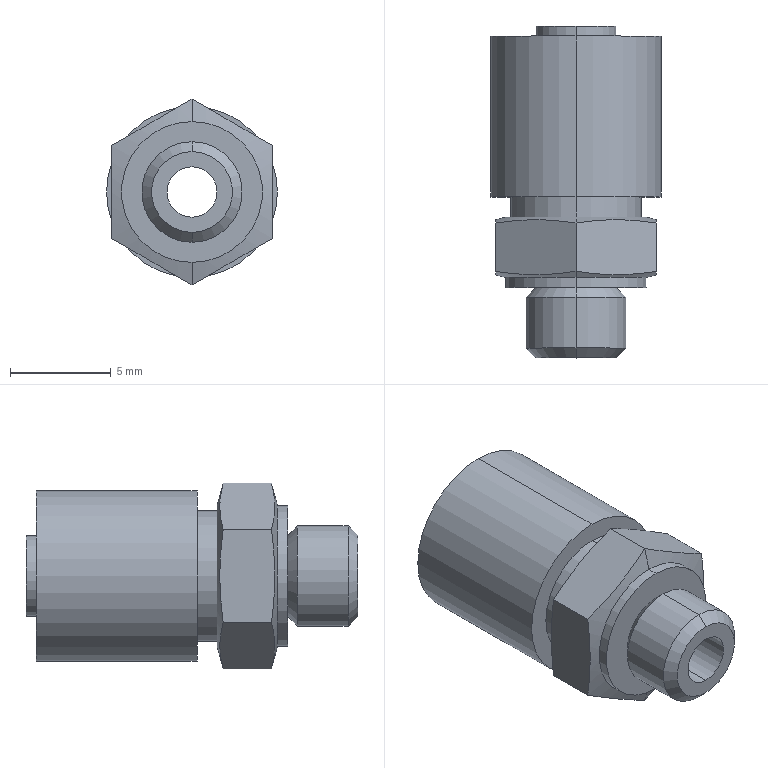Part | SolidWorks | features BaseBody 1 | 1 solid | 32 faces | box 8.5 x 16.5 x 9.238 mm | volume 659.616 mm3 | plane 12 | cylinder 12 | cone 8 | commonest cylinder face diameters 2.5 x2 4 x2 5 x2 6.5 x2 7 x2 8.5 x2
STEP:
#1=CARTESIAN_POINT('',(0.,16.5,-1.25));
#2=VERTEX_POINT('',#1);
#3=CARTESIAN_POINT('',(0.,16.5,1.25));
#4=VERTEX_POINT('',#3);
#5=CARTESIAN_POINT('',(0.,16.5,0.));
#6=DIRECTION('',(0.,-1.,0.));
#7=DIRECTION('',(0.,0.,-1.));
#8=AXIS2_PLACEMENT_3D('',#5,#6,#7);
#9=CIRCLE('',#8,1.25);
#10=EDGE_CURVE('',#2,#4,#9,.T.);
#11=ORIENTED_EDGE('',*,*,#10,.T.);
#12=CARTESIAN_POINT('',(0.,16.5,0.));
#13=DIRECTION('',(0.,-1.,0.));
#14=DIRECTION('',(0.,0.,-1.));
#15=AXIS2_PLACEMENT_3D('',#12,#13,#14);
#16=CIRCLE('',#15,1.25);
#17=EDGE_CURVE('',#4,#2,#16,.T.);
#18=ORIENTED_EDGE('',*,*,#17,.T.);
#19=EDGE_LOOP('',(#11,#18));
#20=FACE_BOUND('',#19,.T.);
#21=CARTESIAN_POINT('',(0.,16.5,-2.));
#22=VERTEX_POINT('',#21);
#23=CARTESIAN_POINT('',(0.,16.5,2.));
#24=VERTEX_POINT('',#23);
#25=CARTESIAN_POINT('',(0.,16.5,0.));
#26=DIRECTION('',(0.,-1.,0.));
#27=DIRECTION('',(0.,0.,-1.));
#28=AXIS2_PLACEMENT_3D('',#25,#26,#27);
#29=CIRCLE('',#28,2.);
#30=EDGE_CURVE('',#22,#24,#29,.T.);
#31=ORIENTED_EDGE('',*,*,#30,.F.);
#32=CARTESIAN_POINT('',(0.,16.5,0.));
#33=DIRECTION('',(0.,-1.,0.));
#34=DIRECTION('',(0.,0.,-1.));
#35=AXIS2_PLACEMENT_3D('',#32,#33,#34);
#36=CIRCLE('',#35,2.);
#37=EDGE_CURVE('',#24,#22,#36,.T.);
#38=ORIENTED_EDGE('',*,*,#37,.F.);
#39=EDGE_LOOP('',(#31,#38));
#40=FACE_OUTER_BOUND('',#39,.T.);
#41=CARTESIAN_POINT('',(2.,16.5,0.));
#42=DIRECTION('',(0.,1.,0.));
#43=DIRECTION('',(1.,0.,0.));
#44=AXIS2_PLACEMENT_3D('',#41,#42,#43);
#45=PLANE('',#44);
#46=ADVANCED_FACE('',(#20,#40),#45,.T.);
#47=CARTESIAN_POINT('',(0.,0.,1.25));
#48=VERTEX_POINT('',#47);
#49=CARTESIAN_POINT('',(0.,0.,1.25));
#50=DIRECTION('',(0.,-1.,0.));
#51=VECTOR('',#50,1000.);
#52=LINE('',#49,#51);
#53=EDGE_CURVE('',#4,#48,#52,.T.);
#54=ORIENTED_EDGE('',*,*,#53,.F.);
#55=ORIENTED_EDGE('',*,*,#10,.F.);
#56=CARTESIAN_POINT('',(0.,0.,-1.25));
#57=VERTEX_POINT('',#56);
#58=CARTESIAN_POINT('',(0.,0.,-1.25));
#59=DIRECTION('',(0.,-1.,0.));
#60=VECTOR('',#59,1000.);
#61=LINE('',#58,#60);
#62=EDGE_CURVE('',#2,#57,#61,.T.);
#63=ORIENTED_EDGE('',*,*,#62,.T.);
#64=CARTESIAN_POINT('',(0.,0.,0.));
#65=DIRECTION('',(0.,-1.,0.));
#66=DIRECTION('',(0.,0.,-1.));
#67=AXIS2_PLACEMENT_3D('',#64,#65,#66);
#68=CIRCLE('',#67,1.25);
#69=EDGE_CURVE('',#57,#48,#68,.T.);
#70=ORIENTED_EDGE('',*,*,#69,.T.);
#71=EDGE_LOOP('',(#54,#55,#63,#70));
#72=FACE_OUTER_BOUND('',#71,.T.);
#73=CARTESIAN_POINT('',(0.,0.,0.));
#74=DIRECTION('',(0.,-1.,0.));
#75=DIRECTION('',(0.,0.,-1.));
#76=AXIS2_PLACEMENT_3D('',#73,#74,#75);
#77=CYLINDRICAL_SURFACE('',#76,1.25);
#78=ADVANCED_FACE('',(#72),#77,.F.);
#79=ORIENTED_EDGE('',*,*,#69,.F.);
#80=CARTESIAN_POINT('',(0.,0.,0.));
#81=DIRECTION('',(0.,-1.,0.));
#82=DIRECTION('',(0.,0.,-1.));
#83=AXIS2_PLACEMENT_3D('',#80,#81,#82);
#84=CIRCLE('',#83,1.25);
#85=EDGE_CURVE('',#48,#57,#84,.T.);
#86=ORIENTED_EDGE('',*,*,#85,.F.);
#87=EDGE_LOOP('',(#79,#86));
#88=FACE_BOUND('',#87,.T.);
#89=CARTESIAN_POINT('',(0.,0.,2.01));
#90=VERTEX_POINT('',#89);
#91=CARTESIAN_POINT('',(0.,0.,-2.01));
#92=VERTEX_POINT('',#91);
#93=CARTESIAN_POINT('',(0.,0.,0.));
#94=DIRECTION('',(0.,-1.,0.));
#95=DIRECTION('',(0.,0.,-1.));
#96=AXIS2_PLACEMENT_3D('',#93,#94,#95);
#97=CIRCLE('',#96,2.01);
#98=EDGE_CURVE('',#90,#92,#97,.T.);
#99=ORIENTED_EDGE('',*,*,#98,.T.);
#100=CARTESIAN_POINT('',(0.,0.,0.));
#101=DIRECTION('',(0.,-1.,0.));
#102=DIRECTION('',(0.,0.,-1.));
#103=AXIS2_PLACEMENT_3D('',#100,#101,#102);
#104=CIRCLE('',#103,2.01);
#105=EDGE_CURVE('',#92,#90,#104,.T.);
#106=ORIENTED_EDGE('',*,*,#105,.T.);
#107=EDGE_LOOP('',(#99,#106));
#108=FACE_OUTER_BOUND('',#107,.T.);
#109=CARTESIAN_POINT('',(1.25,0.,0.));
#110=DIRECTION('',(0.,-1.,0.));
#111=DIRECTION('',(0.,0.,-1.));
#112=AXIS2_PLACEMENT_3D('',#109,#110,#111);
#113=PLANE('',#112);
#114=ADVANCED_FACE('',(#88,#108),#113,.T.);
#115=CARTESIAN_POINT('',(0.,0.4905,-2.5));
#116=VERTEX_POINT('',#115);
#117=CARTESIAN_POINT('',(0.,0.,-2.01));
#118=DIRECTION('',(0.,0.7071,-0.7071));
#119=VECTOR('',#118,1000.);
#120=LINE('',#117,#119);
#121=EDGE_CURVE('',#92,#116,#120,.T.);
#122=ORIENTED_EDGE('',*,*,#121,.F.);
#123=ORIENTED_EDGE('',*,*,#98,.F.);
#124=CARTESIAN_POINT('',(0.,0.4905,2.5));
#125=VERTEX_POINT('',#124);
#126=CARTESIAN_POINT('',(0.,0.,2.01));
#127=DIRECTION('',(0.,0.7071,0.7071));
#128=VECTOR('',#127,1000.);
#129=LINE('',#126,#128);
#130=EDGE_CURVE('',#90,#125,#129,.T.);
#131=ORIENTED_EDGE('',*,*,#130,.T.);
#132=CARTESIAN_POINT('',(0.,0.4905,0.));
#133=DIRECTION('',(0.,-1.,0.));
#134=DIRECTION('',(0.,0.,-1.));
#135=AXIS2_PLACEMENT_3D('',#132,#133,#134);
#136=CIRCLE('',#135,2.5);
#137=EDGE_CURVE('',#125,#116,#136,.T.);
#138=ORIENTED_EDGE('',*,*,#137,.T.);
#139=EDGE_LOOP('',(#122,#123,#131,#138));
#140=FACE_OUTER_BOUND('',#139,.T.);
#141=CARTESIAN_POINT('',(0.,0.,0.));
#142=DIRECTION('',(0.,1.,0.));
#143=DIRECTION('',(0.,0.,1.));
#144=AXIS2_PLACEMENT_3D('',#141,#142,#143);
#145=CONICAL_SURFACE('',#144,2.01,0.7854);
#146=ADVANCED_FACE('',(#140),#145,.T.);
#147=CARTESIAN_POINT('',(0.,3.01,2.5));
#148=VERTEX_POINT('',#147);
#149=CARTESIAN_POINT('',(0.,0.,2.5));
#150=DIRECTION('',(0.,-1.,0.));
#151=VECTOR('',#150,1000.);
#152=LINE('',#149,#151);
#153=EDGE_CURVE('',#148,#125,#152,.T.);
#154=ORIENTED_EDGE('',*,*,#153,.F.);
#155=CARTESIAN_POINT('',(0.,3.01,-2.5));
#156=VERTEX_POINT('',#155);
#157=CARTESIAN_POINT('',(0.,3.01,0.));
#158=DIRECTION('',(0.,-1.,0.));
#159=DIRECTION('',(0.,0.,-1.));
#160=AXIS2_PLACEMENT_3D('',#157,#158,#159);
#161=CIRCLE('',#160,2.5);
#162=EDGE_CURVE('',#148,#156,#161,.T.);
#163=ORIENTED_EDGE('',*,*,#162,.T.);
#164=CARTESIAN_POINT('',(0.,0.,-2.5));
#165=DIRECTION('',(0.,-1.,0.));
#166=VECTOR('',#165,1000.);
#167=LINE('',#164,#166);
#168=EDGE_CURVE('',#156,#116,#167,.T.);
#169=ORIENTED_EDGE('',*,*,#168,.T.);
#170=ORIENTED_EDGE('',*,*,#137,.F.);
#171=EDGE_LOOP('',(#154,#163,#169,#170));
#172=FACE_OUTER_BOUND('',#171,.T.);
#173=CARTESIAN_POINT('',(0.,0.,0.));
#174=DIRECTION('',(0.,-1.,0.));
#175=DIRECTION('',(0.,0.,-1.));
#176=AXIS2_PLACEMENT_3D('',#173,#174,#175);
#177=CYLINDRICAL_SURFACE('',#176,2.5);
#178=ADVANCED_FACE('',(#172),#177,.T.);
#179=CARTESIAN_POINT('',(0.,3.5,2.01));
#180=VERTEX_POINT('',#179);
#181=CARTESIAN_POINT('',(0.,3.01,2.5));
#182=DIRECTION('',(0.,-0.7071,0.7071));
#183=VECTOR('',#182,1000.);
#184=LINE('',#181,#183);
#185=EDGE_CURVE('',#180,#148,#184,.T.);
#186=ORIENTED_EDGE('',*,*,#185,.F.);
#187=CARTESIAN_POINT('',(0.,3.5,-2.01));
#188=VERTEX_POINT('',#187);
#189=CARTESIAN_POINT('',(0.,3.5,0.));
#190=DIRECTION('',(0.,-1.,0.));
#191=DIRECTION('',(0.,0.,-1.));
#192=AXIS2_PLACEMENT_3D('',#189,#190,#191);
#193=CIRCLE('',#192,2.01);
#194=EDGE_CURVE('',#180,#188,#193,.T.);
#195=ORIENTED_EDGE('',*,*,#194,.T.);
#196=CARTESIAN_POINT('',(0.,3.01,-2.5));
#197=DIRECTION('',(0.,-0.7071,-0.7071));
#198=VECTOR('',#197,1000.);
#199=LINE('',#196,#198);
#200=EDGE_CURVE('',#188,#156,#199,.T.);
#201=ORIENTED_EDGE('',*,*,#200,.T.);
#202=ORIENTED_EDGE('',*,*,#162,.F.);
#203=EDGE_LOOP('',(#186,#195,#201,#202));
#204=FACE_OUTER_BOUND('',#203,.T.);
#205=CARTESIAN_POINT('',(0.,3.01,0.));
#206=DIRECTION('',(0.,-1.,0.));
#207=DIRECTION('',(0.,0.,-1.));
#208=AXIS2_PLACEMENT_3D('',#205,#206,#207);
#209=CONICAL_SURFACE('',#208,2.5,0.7854);
#210=ADVANCED_FACE('',(#204),#209,.T.);
#211=CARTESIAN_POINT('',(0.,3.5,0.));
#212=DIRECTION('',(0.,-1.,0.));
#213=DIRECTION('',(0.,0.,-1.));
#214=AXIS2_PLACEMENT_3D('',#211,#212,#213);
#215=CIRCLE('',#214,2.01);
#216=EDGE_CURVE('',#188,#180,#215,.T.);
#217=ORIENTED_EDGE('',*,*,#216,.F.);
#218=ORIENTED_EDGE('',*,*,#194,.F.);
#219=EDGE_LOOP('',(#217,#218));
#220=FACE_BOUND('',#219,.T.);
#221=CARTESIAN_POINT('',(0.,3.5,-3.5));
#222=VERTEX_POINT('',#221);
#223=CARTESIAN_POINT('',(0.,3.5,3.5));
#224=VERTEX_POINT('',#223);
#225=CARTESIAN_POINT('',(0.,3.5,0.));
#226=DIRECTION('',(0.,-1.,0.));
#227=DIRECTION('',(0.,0.,-1.));
#228=AXIS2_PLACEMENT_3D('',#225,#226,#227);
#229=CIRCLE('',#228,3.5);
#230=EDGE_CURVE('',#222,#224,#229,.T.);
#231=ORIENTED_EDGE('',*,*,#230,.T.);
#232=CARTESIAN_POINT('',(0.,3.5,0.));
#233=DIRECTION('',(0.,-1.,0.));
#234=DIRECTION('',(0.,0.,-1.));
#235=AXIS2_PLACEMENT_3D('',#232,#233,#234);
#236=CIRCLE('',#235,3.5);
#237=EDGE_CURVE('',#224,#222,#236,.T.);
#238=ORIENTED_EDGE('',*,*,#237,.T.);
#239=EDGE_LOOP('',(#231,#238));
#240=FACE_OUTER_BOUND('',#239,.T.);
#241=CARTESIAN_POINT('',(2.01,3.5,0.));
#242=DIRECTION('',(0.,-1.,0.));
#243=DIRECTION('',(0.,0.,-1.));
#244=AXIS2_PLACEMENT_3D('',#241,#242,#243);
#245=PLANE('',#244);
#246=ADVANCED_FACE('',(#220,#240),#245,.T.);
#247=CARTESIAN_POINT('',(0.,4.,3.5));
#248=VERTEX_POINT('',#247);
#249=CARTESIAN_POINT('',(0.,0.,3.5));
#250=DIRECTION('',(0.,-1.,0.));
#251=VECTOR('',#250,1000.);
#252=LINE('',#249,#251);
#253=EDGE_CURVE('',#248,#224,#252,.T.);
#254=ORIENTED_EDGE('',*,*,#253,.F.);
#255=CARTESIAN_POINT('',(0.,4.,-3.5));
#256=VERTEX_POINT('',#255);
#257=CARTESIAN_POINT('',(0.,4.,0.));
#258=DIRECTION('',(0.,-1.,0.));
#259=DIRECTION('',(0.,0.,-1.));
#260=AXIS2_PLACEMENT_3D('',#257,#258,#259);
#261=CIRCLE('',#260,3.5);
#262=EDGE_CURVE('',#248,#256,#261,.T.);
#263=ORIENTED_EDGE('',*,*,#262,.T.);
#264=CARTESIAN_POINT('',(0.,0.,-3.5));
#265=DIRECTION('',(0.,-1.,0.));
#266=VECTOR('',#265,1000.);
#267=LINE('',#264,#266);
#268=EDGE_CURVE('',#256,#222,#267,.T.);
#269=ORIENTED_EDGE('',*,*,#268,.T.);
#270=ORIENTED_EDGE('',*,*,#237,.F.);
#271=EDGE_LOOP('',(#254,#263,#269,#270));
#272=FACE_OUTER_BOUND('',#271,.T.);
#273=CARTESIAN_POINT('',(0.,0.,0.));
#274=DIRECTION('',(0.,-1.,0.));
#275=DIRECTION('',(0.,0.,-1.));
#276=AXIS2_PLACEMENT_3D('',#273,#274,#275);
#277=CYLINDRICAL_SURFACE('',#276,3.5);
#278=ADVANCED_FACE('',(#272),#277,.T.);
#279=CARTESIAN_POINT('',(0.,4.3,-4.619));
#280=VERTEX_POINT('',#279);
#281=CARTESIAN_POINT('',(0.,4.,-3.5));
#282=DIRECTION('',(0.,0.2588,-0.9659));
#283=VECTOR('',#282,1000.);
#284=LINE('',#281,#283);
#285=EDGE_CURVE('',#256,#280,#284,.T.);
#286=ORIENTED_EDGE('',*,*,#285,.F.);
#287=ORIENTED_EDGE('',*,*,#262,.F.);
#288=CARTESIAN_POINT('',(0.,4.3,4.619));
#289=VERTEX_POINT('',#288);
#290=CARTESIAN_POINT('',(0.,4.,3.5));
#291=DIRECTION('',(0.,0.2588,0.9659));
#292=VECTOR('',#291,1000.);
#293=LINE('',#290,#292);
#294=EDGE_CURVE('',#248,#289,#293,.T.);
#295=ORIENTED_EDGE('',*,*,#294,.T.);
#296=CARTESIAN_POINT('',(-4.,4.3,2.309));
#297=VERTEX_POINT('',#296);
#298=CARTESIAN_POINT('',(-4.,4.3,2.309));
#299=CARTESIAN_POINT('',(-3.286,4.189,2.722));
#300=CARTESIAN_POINT('',(-2.618,4.134,3.107));
#301=CARTESIAN_POINT('',(-1.382,4.134,3.821));
#302=CARTESIAN_POINT('',(-0.7149,4.189,4.206));
#303=CARTESIAN_POINT('',(0.,4.3,4.619));
#304=B_SPLINE_CURVE_WITH_KNOTS('',3,(#298,#299,#300,#301,#302,#303),.UNSPECIFIED.,.F.,.F.,(4,2,4),(0.,0.5,1.),.UNSPECIFIED.);
#305=EDGE_CURVE('',#297,#289,#304,.T.);
#306=ORIENTED_EDGE('',*,*,#305,.F.);
#307=CARTESIAN_POINT('',(-4.,4.3,-2.309));
#308=VERTEX_POINT('',#307);
#309=CARTESIAN_POINT('',(-4.,4.3,-2.309));
#310=CARTESIAN_POINT('',(-4.,4.245,-1.899));
#311=CARTESIAN_POINT('',(-4.,4.183,-1.304));
#312=CARTESIAN_POINT('',(-4.,4.146,-0.6473));
#313=CARTESIAN_POINT('',(-4.,4.138,-0.3741));
#314=CARTESIAN_POINT('',(-4.,4.135,-0.1937));
#315=CARTESIAN_POINT('',(-4.,4.134,-0.1062));
#316=CARTESIAN_POINT('',(-4.,4.134,0.7059));
#317=CARTESIAN_POINT('',(-4.,4.189,1.481));
#318=CARTESIAN_POINT('',(-4.,4.3,2.309));
#319=B_SPLINE_CURVE_WITH_KNOTS('',3,(#309,#310,#311,#312,#313,#314,#315,#316,#317,#318),.UNSPECIFIED.,.F.,.F.,(4,1,1,2,2,4),(0.,0.25,0.375,0.4375,0.5,1.),.UNSPECIFIED.);
#320=EDGE_CURVE('',#308,#297,#319,.T.);
#321=ORIENTED_EDGE('',*,*,#320,.F.);
#322=CARTESIAN_POINT('',(0.,4.3,-4.619));
#323=CARTESIAN_POINT('',(-0.7142,4.189,-4.206));
#324=CARTESIAN_POINT('',(-1.382,4.134,-3.821));
#325=CARTESIAN_POINT('',(-2.618,4.134,-3.107));
#326=CARTESIAN_POINT('',(-3.285,4.189,-2.722));
#327=CARTESIAN_POINT('',(-4.,4.3,-2.309));
#328=B_SPLINE_CURVE_WITH_KNOTS('',3,(#322,#323,#324,#325,#326,#327),.UNSPECIFIED.,.F.,.F.,(4,2,4),(0.,0.5,1.),.UNSPECIFIED.);
#329=EDGE_CURVE('',#280,#308,#328,.T.);
#330=ORIENTED_EDGE('',*,*,#329,.F.);
#331=EDGE_LOOP('',(#286,#287,#295,#306,#321,#330));
#332=FACE_OUTER_BOUND('',#331,.T.);
#333=CARTESIAN_POINT('',(0.,4.,0.));
#334=DIRECTION('',(0.,1.,0.));
#335=DIRECTION('',(0.,0.,1.));
#336=AXIS2_PLACEMENT_3D('',#333,#334,#335);
#337=CONICAL_SURFACE('',#336,3.5,1.309);
#338=ADVANCED_FACE('',(#332),#337,.T.);
#339=CARTESIAN_POINT('',(0.,7.,3.5));
#340=VERTEX_POINT('',#339);
#341=CARTESIAN_POINT('',(0.,6.7,4.619));
#342=VERTEX_POINT('',#341);
#343=CARTESIAN_POINT('',(0.,5.794,8.));
#344=DIRECTION('',(0.,-0.2588,0.9659));
#345=VECTOR('',#344,1000.);
#346=LINE('',#343,#345);
#347=EDGE_CURVE('',#340,#342,#346,.T.);
#348=ORIENTED_EDGE('',*,*,#347,.F.);
#349=CARTESIAN_POINT('',(0.,7.,-3.5));
#350=VERTEX_POINT('',#349);
#351=CARTESIAN_POINT('',(0.,7.,0.));
#352=DIRECTION('',(0.,-1.,0.));
#353=DIRECTION('',(0.,0.,-1.));
#354=AXIS2_PLACEMENT_3D('',#351,#352,#353);
#355=CIRCLE('',#354,3.5);
#356=EDGE_CURVE('',#340,#350,#355,.T.);
#357=ORIENTED_EDGE('',*,*,#356,.T.);
#358=CARTESIAN_POINT('',(0.,6.7,-4.619));
#359=VERTEX_POINT('',#358);
#360=CARTESIAN_POINT('',(0.,5.794,-8.));
#361=DIRECTION('',(0.,-0.2588,-0.9659));
#362=VECTOR('',#361,1000.);
#363=LINE('',#360,#362);
#364=EDGE_CURVE('',#350,#359,#363,.T.);
#365=ORIENTED_EDGE('',*,*,#364,.T.);
#366=CARTESIAN_POINT('',(-4.,6.7,-2.309));
#367=VERTEX_POINT('',#366);
#368=CARTESIAN_POINT('',(-4.,6.7,-2.309));
#369=CARTESIAN_POINT('',(-3.286,6.811,-2.722));
#370=CARTESIAN_POINT('',(-2.618,6.866,-3.107));
#371=CARTESIAN_POINT('',(-1.382,6.866,-3.821));
#372=CARTESIAN_POINT('',(-0.7149,6.811,-4.206));
#373=CARTESIAN_POINT('',(0.,6.7,-4.619));
#374=B_SPLINE_CURVE_WITH_KNOTS('',3,(#368,#369,#370,#371,#372,#373),.UNSPECIFIED.,.F.,.F.,(4,2,4),(0.,0.5,1.),.UNSPECIFIED.);
#375=EDGE_CURVE('',#367,#359,#374,.T.);
#376=ORIENTED_EDGE('',*,*,#375,.F.);
#377=CARTESIAN_POINT('',(-4.,6.7,2.309));
#378=VERTEX_POINT('',#377);
#379=CARTESIAN_POINT('',(-4.,6.7,2.309));
#380=CARTESIAN_POINT('',(-4.,6.755,1.899));
#381=CARTESIAN_POINT('',(-4.,6.817,1.304));
#382=CARTESIAN_POINT('',(-4.,6.854,0.6473));
#383=CARTESIAN_POINT('',(-4.,6.862,0.3741));
#384=CARTESIAN_POINT('',(-4.,6.865,0.1937));
#385=CARTESIAN_POINT('',(-4.,6.866,0.1062));
#386=CARTESIAN_POINT('',(-4.,6.866,-0.7059));
#387=CARTESIAN_POINT('',(-4.,6.811,-1.481));
#388=CARTESIAN_POINT('',(-4.,6.7,-2.309));
#389=B_SPLINE_CURVE_WITH_KNOTS('',3,(#379,#380,#381,#382,#383,#384,#385,#386,#387,#388),.UNSPECIFIED.,.F.,.F.,(4,1,1,2,2,4),(0.,0.25,0.375,0.4375,0.5,1.),.UNSPECIFIED.);
#390=EDGE_CURVE('',#378,#367,#389,.T.);
#391=ORIENTED_EDGE('',*,*,#390,.F.);
#392=CARTESIAN_POINT('',(0.,6.7,4.619));
#393=CARTESIAN_POINT('',(-0.7142,6.811,4.206));
#394=CARTESIAN_POINT('',(-1.382,6.866,3.821));
#395=CARTESIAN_POINT('',(-2.618,6.866,3.107));
#396=CARTESIAN_POINT('',(-3.285,6.811,2.722));
#397=CARTESIAN_POINT('',(-4.,6.7,2.309));
#398=B_SPLINE_CURVE_WITH_KNOTS('',3,(#392,#393,#394,#395,#396,#397),.UNSPECIFIED.,.F.,.F.,(4,2,4),(0.,0.5,1.),.UNSPECIFIED.);
#399=EDGE_CURVE('',#342,#378,#398,.T.);
#400=ORIENTED_EDGE('',*,*,#399,.F.);
#401=EDGE_LOOP('',(#348,#357,#365,#376,#391,#400));
#402=FACE_OUTER_BOUND('',#401,.T.);
#403=CARTESIAN_POINT('',(0.,5.794,0.));
#404=DIRECTION('',(0.,-1.,0.));
#405=DIRECTION('',(0.,0.,-1.));
#406=AXIS2_PLACEMENT_3D('',#403,#404,#405);
#407=CONICAL_SURFACE('',#406,8.,1.309);
#408=ADVANCED_FACE('',(#402),#407,.T.);
#409=CARTESIAN_POINT('',(0.,7.,-3.25));
#410=VERTEX_POINT('',#409);
#411=CARTESIAN_POINT('',(0.,7.,3.25));
#412=VERTEX_POINT('',#411);
#413=CARTESIAN_POINT('',(0.,7.,0.));
#414=DIRECTION('',(0.,-1.,0.));
#415=DIRECTION('',(0.,0.,-1.));
#416=AXIS2_PLACEMENT_3D('',#413,#414,#415);
#417=CIRCLE('',#416,3.25);
#418=EDGE_CURVE('',#410,#412,#417,.T.);
#419=ORIENTED_EDGE('',*,*,#418,.T.);
#420=CARTESIAN_POINT('',(0.,7.,0.));
#421=DIRECTION('',(0.,-1.,0.));
#422=DIRECTION('',(0.,0.,-1.));
#423=AXIS2_PLACEMENT_3D('',#420,#421,#422);
#424=CIRCLE('',#423,3.25);
#425=EDGE_CURVE('',#412,#410,#424,.T.);
#426=ORIENTED_EDGE('',*,*,#425,.T.);
#427=EDGE_LOOP('',(#419,#426));
#428=FACE_BOUND('',#427,.T.);
#429=CARTESIAN_POINT('',(0.,7.,0.));
#430=DIRECTION('',(0.,-1.,0.));
#431=DIRECTION('',(0.,0.,-1.));
#432=AXIS2_PLACEMENT_3D('',#429,#430,#431);
#433=CIRCLE('',#432,3.5);
#434=EDGE_CURVE('',#350,#340,#433,.T.);
#435=ORIENTED_EDGE('',*,*,#434,.F.);
#436=ORIENTED_EDGE('',*,*,#356,.F.);
#437=EDGE_LOOP('',(#435,#436));
#438=FACE_OUTER_BOUND('',#437,.T.);
#439=CARTESIAN_POINT('',(3.5,7.,0.));
#440=DIRECTION('',(0.,1.,0.));
#441=DIRECTION('',(1.,0.,0.));
#442=AXIS2_PLACEMENT_3D('',#439,#440,#441);
#443=PLANE('',#442);
#444=ADVANCED_FACE('',(#428,#438),#443,.T.);
#445=CARTESIAN_POINT('',(0.,8.,3.25));
#446=VERTEX_POINT('',#445);
#447=CARTESIAN_POINT('',(0.,0.,3.25));
#448=DIRECTION('',(0.,-1.,0.));
#449=VECTOR('',#448,1000.);
#450=LINE('',#447,#449);
#451=EDGE_CURVE('',#446,#412,#450,.T.);
#452=ORIENTED_EDGE('',*,*,#451,.F.);
#453=CARTESIAN_POINT('',(0.,8.,-3.25));
#454=VERTEX_POINT('',#453);
#455=CARTESIAN_POINT('',(0.,8.,0.));
#456=DIRECTION('',(0.,-1.,0.));
#457=DIRECTION('',(0.,0.,-1.));
#458=AXIS2_PLACEMENT_3D('',#455,#456,#457);
#459=CIRCLE('',#458,3.25);
#460=EDGE_CURVE('',#446,#454,#459,.T.);
#461=ORIENTED_EDGE('',*,*,#460,.T.);
#462=CARTESIAN_POINT('',(0.,0.,-3.25));
#463=DIRECTION('',(0.,-1.,0.));
#464=VECTOR('',#463,1000.);
#465=LINE('',#462,#464);
#466=EDGE_CURVE('',#454,#410,#465,.T.);
#467=ORIENTED_EDGE('',*,*,#466,.T.);
#468=ORIENTED_EDGE('',*,*,#425,.F.);
#469=EDGE_LOOP('',(#452,#461,#467,#468));
#470=FACE_OUTER_BOUND('',#469,.T.);
#471=CARTESIAN_POINT('',(0.,0.,0.));
#472=DIRECTION('',(0.,-1.,0.));
#473=DIRECTION('',(0.,0.,-1.));
#474=AXIS2_PLACEMENT_3D('',#471,#472,#473);
#475=CYLINDRICAL_SURFACE('',#474,3.25);
#476=ADVANCED_FACE('',(#470),#475,.T.);
#477=CARTESIAN_POINT('',(0.,8.,0.));
#478=DIRECTION('',(0.,-1.,0.));
#479=DIRECTION('',(0.,0.,-1.));
#480=AXIS2_PLACEMENT_3D('',#477,#478,#479);
#481=CIRCLE('',#480,3.25);
#482=EDGE_CURVE('',#454,#446,#481,.T.);
#483=ORIENTED_EDGE('',*,*,#482,.F.);
#484=ORIENTED_EDGE('',*,*,#460,.F.);
#485=EDGE_LOOP('',(#483,#484));
#486=FACE_BOUND('',#485,.T.);
#487=CARTESIAN_POINT('',(0.,8.,-4.25));
#488=VERTEX_POINT('',#487);
#489=CARTESIAN_POINT('',(0.,8.,4.25));
#490=VERTEX_POINT('',#489);
#491=CARTESIAN_POINT('',(0.,8.,0.));
#492=DIRECTION('',(0.,-1.,0.));
#493=DIRECTION('',(0.,0.,-1.));
#494=AXIS2_PLACEMENT_3D('',#491,#492,#493);
#495=CIRCLE('',#494,4.25);
#496=EDGE_CURVE('',#488,#490,#495,.T.);
#497=ORIENTED_EDGE('',*,*,#496,.T.);
#498=CARTESIAN_POINT('',(0.,8.,0.));
#499=DIRECTION('',(0.,-1.,0.));
#500=DIRECTION('',(0.,0.,-1.));
#501=AXIS2_PLACEMENT_3D('',#498,#499,#500);
#502=CIRCLE('',#501,4.25);
#503=EDGE_CURVE('',#490,#488,#502,.T.);
#504=ORIENTED_EDGE('',*,*,#503,.T.);
#505=EDGE_LOOP('',(#497,#504));
#506=FACE_OUTER_BOUND('',#505,.T.);
#507=CARTESIAN_POINT('',(3.25,8.,0.));
#508=DIRECTION('',(0.,-1.,0.));
#509=DIRECTION('',(0.,0.,-1.));
#510=AXIS2_PLACEMENT_3D('',#507,#508,#509);
#511=PLANE('',#510);
#512=ADVANCED_FACE('',(#486,#506),#511,.T.);
#513=CARTESIAN_POINT('',(0.,16.,4.25));
#514=VERTEX_POINT('',#513);
#515=CARTESIAN_POINT('',(0.,0.,4.25));
#516=DIRECTION('',(0.,-1.,0.));
#517=VECTOR('',#516,1000.);
#518=LINE('',#515,#517);
#519=EDGE_CURVE('',#514,#490,#518,.T.);
#520=ORIENTED_EDGE('',*,*,#519,.F.);
#521=CARTESIAN_POINT('',(0.,16.,-4.25));
#522=VERTEX_POINT('',#521);
#523=CARTESIAN_POINT('',(0.,16.,0.));
#524=DIRECTION('',(0.,-1.,0.));
#525=DIRECTION('',(0.,0.,-1.));
#526=AXIS2_PLACEMENT_3D('',#523,#524,#525);
#527=CIRCLE('',#526,4.25);
#528=EDGE_CURVE('',#514,#522,#527,.T.);
#529=ORIENTED_EDGE('',*,*,#528,.T.);
#530=CARTESIAN_POINT('',(0.,0.,-4.25));
#531=DIRECTION('',(0.,-1.,0.));
#532=VECTOR('',#531,1000.);
#533=LINE('',#530,#532);
#534=EDGE_CURVE('',#522,#488,#533,.T.);
#535=ORIENTED_EDGE('',*,*,#534,.T.);
#536=ORIENTED_EDGE('',*,*,#503,.F.);
#537=EDGE_LOOP('',(#520,#529,#535,#536));
#538=FACE_OUTER_BOUND('',#537,.T.);
#539=CARTESIAN_POINT('',(0.,0.,0.));
#540=DIRECTION('',(0.,-1.,0.));
#541=DIRECTION('',(0.,0.,-1.));
#542=AXIS2_PLACEMENT_3D('',#539,#540,#541);
#543=CYLINDRICAL_SURFACE('',#542,4.25);
#544=ADVANCED_FACE('',(#538),#543,.T.);
#545=CARTESIAN_POINT('',(0.,16.,-2.));
#546=VERTEX_POINT('',#545);
#547=CARTESIAN_POINT('',(0.,16.,2.));
#548=VERTEX_POINT('',#547);
#549=CARTESIAN_POINT('',(0.,16.,0.));
#550=DIRECTION('',(0.,-1.,0.));
#551=DIRECTION('',(0.,0.,-1.));
#552=AXIS2_PLACEMENT_3D('',#549,#550,#551);
#553=CIRCLE('',#552,2.);
#554=EDGE_CURVE('',#546,#548,#553,.T.);
#555=ORIENTED_EDGE('',*,*,#554,.T.);
#556=CARTESIAN_POINT('',(0.,16.,0.));
#557=DIRECTION('',(0.,-1.,0.));
#558=DIRECTION('',(0.,0.,-1.));
#559=AXIS2_PLACEMENT_3D('',#556,#557,#558);
#560=CIRCLE('',#559,2.);
#561=EDGE_CURVE('',#548,#546,#560,.T.);
#562=ORIENTED_EDGE('',*,*,#561,.T.);
#563=EDGE_LOOP('',(#555,#562));
#564=FACE_BOUND('',#563,.T.);
#565=CARTESIAN_POINT('',(0.,16.,0.));
#566=DIRECTION('',(0.,-1.,0.));
#567=DIRECTION('',(0.,0.,-1.));
#568=AXIS2_PLACEMENT_3D('',#565,#566,#567);
#569=CIRCLE('',#568,4.25);
#570=EDGE_CURVE('',#522,#514,#569,.T.);
#571=ORIENTED_EDGE('',*,*,#570,.F.);
#572=ORIENTED_EDGE('',*,*,#528,.F.);
#573=EDGE_LOOP('',(#571,#572));
#574=FACE_OUTER_BOUND('',#573,.T.);
#575=CARTESIAN_POINT('',(4.25,16.,0.));
#576=DIRECTION('',(0.,1.,0.));
#577=DIRECTION('',(1.,0.,0.));
#578=AXIS2_PLACEMENT_3D('',#575,#576,#577);
#579=PLANE('',#578);
#580=ADVANCED_FACE('',(#564,#574),#579,.T.);
#581=CARTESIAN_POINT('',(0.,0.,2.));
#582=DIRECTION('',(0.,-1.,0.));
#583=VECTOR('',#582,1000.);
#584=LINE('',#581,#583);
#585=EDGE_CURVE('',#24,#548,#584,.T.);
#586=ORIENTED_EDGE('',*,*,#585,.F.);
#587=ORIENTED_EDGE('',*,*,#37,.T.);
#588=CARTESIAN_POINT('',(0.,0.,-2.));
#589=DIRECTION('',(0.,-1.,0.));
#590=VECTOR('',#589,1000.);
#591=LINE('',#588,#590);
#592=EDGE_CURVE('',#22,#546,#591,.T.);
#593=ORIENTED_EDGE('',*,*,#592,.T.);
#594=ORIENTED_EDGE('',*,*,#561,.F.);
#595=EDGE_LOOP('',(#586,#587,#593,#594));
#596=FACE_OUTER_BOUND('',#595,.T.);
#597=CARTESIAN_POINT('',(0.,0.,0.));
#598=DIRECTION('',(0.,-1.,0.));
#599=DIRECTION('',(0.,0.,-1.));
#600=AXIS2_PLACEMENT_3D('',#597,#598,#599);
#601=CYLINDRICAL_SURFACE('',#600,2.);
#602=ADVANCED_FACE('',(#596),#601,.T.);
#603=ORIENTED_EDGE('',*,*,#320,.T.);
#604=CARTESIAN_POINT('',(-4.,7.,2.309));
#605=DIRECTION('',(0.,-1.,0.));
#606=VECTOR('',#605,1000.);
#607=LINE('',#604,#606);
#608=EDGE_CURVE('',#378,#297,#607,.T.);
#609=ORIENTED_EDGE('',*,*,#608,.F.);
#610=ORIENTED_EDGE('',*,*,#390,.T.);
#611=CARTESIAN_POINT('',(-4.,7.,-2.309));
#612=DIRECTION('',(0.,-1.,0.));
#613=VECTOR('',#612,1000.);
#614=LINE('',#611,#613);
#615=EDGE_CURVE('',#367,#308,#614,.T.);
#616=ORIENTED_EDGE('',*,*,#615,.T.);
#617=EDGE_LOOP('',(#603,#609,#610,#616));
#618=FACE_OUTER_BOUND('',#617,.T.);
#619=CARTESIAN_POINT('',(-4.,7.,-2.309));
#620=DIRECTION('',(1.,0.,0.));
#621=DIRECTION('',(0.,1.,0.));
#622=AXIS2_PLACEMENT_3D('',#619,#620,#621);
#623=PLANE('',#622);
#624=ADVANCED_FACE('',(#618),#623,.F.);
#625=ORIENTED_EDGE('',*,*,#329,.T.);
#626=ORIENTED_EDGE('',*,*,#615,.F.);
#627=ORIENTED_EDGE('',*,*,#375,.T.);
#628=CARTESIAN_POINT('',(0.,7.,-4.619));
#629=DIRECTION('',(0.,-1.,0.));
#630=VECTOR('',#629,1000.);
#631=LINE('',#628,#630);
#632=EDGE_CURVE('',#359,#280,#631,.T.);
#633=ORIENTED_EDGE('',*,*,#632,.T.);
#634=EDGE_LOOP('',(#625,#626,#627,#633));
#635=FACE_OUTER_BOUND('',#634,.T.);
#636=CARTESIAN_POINT('',(0.,7.,-4.619));
#637=DIRECTION('',(0.5,0.,0.866));
#638=DIRECTION('',(0.,-1.,0.));
#639=AXIS2_PLACEMENT_3D('',#636,#637,#638);
#640=PLANE('',#639);
#641=ADVANCED_FACE('',(#635),#640,.F.);
#642=CARTESIAN_POINT('',(4.,4.3,-2.309));
#643=VERTEX_POINT('',#642);
#644=CARTESIAN_POINT('',(4.,4.3,-2.309));
#645=CARTESIAN_POINT('',(3.286,4.189,-2.722));
#646=CARTESIAN_POINT('',(2.618,4.134,-3.107));
#647=CARTESIAN_POINT('',(1.382,4.134,-3.821));
#648=CARTESIAN_POINT('',(0.7149,4.189,-4.206));
#649=CARTESIAN_POINT('',(0.,4.3,-4.619));
#650=B_SPLINE_CURVE_WITH_KNOTS('',3,(#644,#645,#646,#647,#648,#649),.UNSPECIFIED.,.F.,.F.,(4,2,4),(0.,0.5,1.),.UNSPECIFIED.);
#651=EDGE_CURVE('',#643,#280,#650,.T.);
#652=ORIENTED_EDGE('',*,*,#651,.T.);
#653=ORIENTED_EDGE('',*,*,#632,.F.);
#654=CARTESIAN_POINT('',(4.,6.7,-2.309));
#655=VERTEX_POINT('',#654);
#656=CARTESIAN_POINT('',(0.,6.7,-4.619));
#657=CARTESIAN_POINT('',(0.7142,6.811,-4.206));
#658=CARTESIAN_POINT('',(1.382,6.866,-3.821));
#659=CARTESIAN_POINT('',(2.618,6.866,-3.107));
#660=CARTESIAN_POINT('',(3.285,6.811,-2.722));
#661=CARTESIAN_POINT('',(4.,6.7,-2.309));
#662=B_SPLINE_CURVE_WITH_KNOTS('',3,(#656,#657,#658,#659,#660,#661),.UNSPECIFIED.,.F.,.F.,(4,2,4),(0.,0.5,1.),.UNSPECIFIED.);
#663=EDGE_CURVE('',#359,#655,#662,.T.);
#664=ORIENTED_EDGE('',*,*,#663,.T.);
#665=CARTESIAN_POINT('',(4.,7.,-2.309));
#666=DIRECTION('',(0.,-1.,0.));
#667=VECTOR('',#666,1000.);
#668=LINE('',#665,#667);
#669=EDGE_CURVE('',#655,#643,#668,.T.);
#670=ORIENTED_EDGE('',*,*,#669,.T.);
#671=EDGE_LOOP('',(#652,#653,#664,#670));
#672=FACE_OUTER_BOUND('',#671,.T.);
#673=CARTESIAN_POINT('',(4.,7.,-2.309));
#674=DIRECTION('',(-0.5,0.,0.866));
#675=DIRECTION('',(0.,1.,0.));
#676=AXIS2_PLACEMENT_3D('',#673,#674,#675);
#677=PLANE('',#676);
#678=ADVANCED_FACE('',(#672),#677,.F.);
#679=CARTESIAN_POINT('',(4.,4.3,2.309));
#680=VERTEX_POINT('',#679);
#681=CARTESIAN_POINT('',(4.,4.3,2.309));
#682=CARTESIAN_POINT('',(4.,4.245,1.899));
#683=CARTESIAN_POINT('',(4.,4.183,1.304));
#684=CARTESIAN_POINT('',(4.,4.146,0.6473));
#685=CARTESIAN_POINT('',(4.,4.138,0.3741));
#686=CARTESIAN_POINT('',(4.,4.135,0.1937));
#687=CARTESIAN_POINT('',(4.,4.134,0.1062));
#688=CARTESIAN_POINT('',(4.,4.134,-0.7059));
#689=CARTESIAN_POINT('',(4.,4.189,-1.481));
#690=CARTESIAN_POINT('',(4.,4.3,-2.309));
#691=B_SPLINE_CURVE_WITH_KNOTS('',3,(#681,#682,#683,#684,#685,#686,#687,#688,#689,#690),.UNSPECIFIED.,.F.,.F.,(4,1,1,2,2,4),(0.,0.25,0.375,0.4375,0.5,1.),.UNSPECIFIED.);
#692=EDGE_CURVE('',#680,#643,#691,.T.);
#693=ORIENTED_EDGE('',*,*,#692,.T.);
#694=ORIENTED_EDGE('',*,*,#669,.F.);
#695=CARTESIAN_POINT('',(4.,6.7,2.309));
#696=VERTEX_POINT('',#695);
#697=CARTESIAN_POINT('',(4.,6.7,-2.309));
#698=CARTESIAN_POINT('',(4.,6.755,-1.899));
#699=CARTESIAN_POINT('',(4.,6.817,-1.304));
#700=CARTESIAN_POINT('',(4.,6.854,-0.6473));
#701=CARTESIAN_POINT('',(4.,6.862,-0.3741));
#702=CARTESIAN_POINT('',(4.,6.865,-0.1937));
#703=CARTESIAN_POINT('',(4.,6.866,-0.1062));
#704=CARTESIAN_POINT('',(4.,6.866,0.7059));
#705=CARTESIAN_POINT('',(4.,6.811,1.481));
#706=CARTESIAN_POINT('',(4.,6.7,2.309));
#707=B_SPLINE_CURVE_WITH_KNOTS('',3,(#697,#698,#699,#700,#701,#702,#703,#704,#705,#706),.UNSPECIFIED.,.F.,.F.,(4,1,1,2,2,4),(0.,0.25,0.375,0.4375,0.5,1.),.UNSPECIFIED.);
#708=EDGE_CURVE('',#655,#696,#707,.T.);
#709=ORIENTED_EDGE('',*,*,#708,.T.);
#710=CARTESIAN_POINT('',(4.,7.,2.309));
#711=DIRECTION('',(0.,-1.,0.));
#712=VECTOR('',#711,1000.);
#713=LINE('',#710,#712);
#714=EDGE_CURVE('',#696,#680,#713,.T.);
#715=ORIENTED_EDGE('',*,*,#714,.T.);
#716=EDGE_LOOP('',(#693,#694,#709,#715));
#717=FACE_OUTER_BOUND('',#716,.T.);
#718=CARTESIAN_POINT('',(4.,7.,2.309));
#719=DIRECTION('',(-1.,0.,0.));
#720=DIRECTION('',(0.,0.,1.));
#721=AXIS2_PLACEMENT_3D('',#718,#719,#720);
#722=PLANE('',#721);
#723=ADVANCED_FACE('',(#717),#722,.F.);
#724=CARTESIAN_POINT('',(0.,4.3,4.619));
#725=CARTESIAN_POINT('',(0.7142,4.189,4.206));
#726=CARTESIAN_POINT('',(1.382,4.134,3.821));
#727=CARTESIAN_POINT('',(2.618,4.134,3.107));
#728=CARTESIAN_POINT('',(3.285,4.189,2.722));
#729=CARTESIAN_POINT('',(4.,4.3,2.309));
#730=B_SPLINE_CURVE_WITH_KNOTS('',3,(#724,#725,#726,#727,#728,#729),.UNSPECIFIED.,.F.,.F.,(4,2,4),(0.,0.5,1.),.UNSPECIFIED.);
#731=EDGE_CURVE('',#289,#680,#730,.T.);
#732=ORIENTED_EDGE('',*,*,#731,.T.);
#733=ORIENTED_EDGE('',*,*,#714,.F.);
#734=CARTESIAN_POINT('',(4.,6.7,2.309));
#735=CARTESIAN_POINT('',(3.286,6.811,2.722));
#736=CARTESIAN_POINT('',(2.618,6.866,3.107));
#737=CARTESIAN_POINT('',(1.382,6.866,3.821));
#738=CARTESIAN_POINT('',(0.7149,6.811,4.206));
#739=CARTESIAN_POINT('',(0.,6.7,4.619));
#740=B_SPLINE_CURVE_WITH_KNOTS('',3,(#734,#735,#736,#737,#738,#739),.UNSPECIFIED.,.F.,.F.,(4,2,4),(0.,0.5,1.),.UNSPECIFIED.);
#741=EDGE_CURVE('',#696,#342,#740,.T.);
#742=ORIENTED_EDGE('',*,*,#741,.T.);
#743=CARTESIAN_POINT('',(0.,7.,4.619));
#744=DIRECTION('',(0.,-1.,0.));
#745=VECTOR('',#744,1000.);
#746=LINE('',#743,#745);
#747=EDGE_CURVE('',#342,#289,#746,.T.);
#748=ORIENTED_EDGE('',*,*,#747,.T.);
#749=EDGE_LOOP('',(#732,#733,#742,#748));
#750=FACE_OUTER_BOUND('',#749,.T.);
#751=CARTESIAN_POINT('',(0.,7.,4.619));
#752=DIRECTION('',(-0.5,0.,-0.866));
#753=DIRECTION('',(-0.866,0.,0.5));
#754=AXIS2_PLACEMENT_3D('',#751,#752,#753);
#755=PLANE('',#754);
#756=ADVANCED_FACE('',(#750),#755,.F.);
#757=ORIENTED_EDGE('',*,*,#305,.T.);
#758=ORIENTED_EDGE('',*,*,#747,.F.);
#759=ORIENTED_EDGE('',*,*,#399,.T.);
#760=ORIENTED_EDGE('',*,*,#608,.T.);
#761=EDGE_LOOP('',(#757,#758,#759,#760));
#762=FACE_OUTER_BOUND('',#761,.T.);
#763=CARTESIAN_POINT('',(-4.,7.,2.309));
#764=DIRECTION('',(0.5,0.,-0.866));
#765=DIRECTION('',(0.,-1.,0.));
#766=AXIS2_PLACEMENT_3D('',#763,#764,#765);
#767=PLANE('',#766);
#768=ADVANCED_FACE('',(#762),#767,.F.);
#769=ORIENTED_EDGE('',*,*,#30,.T.);
#770=ORIENTED_EDGE('',*,*,#585,.T.);
#771=ORIENTED_EDGE('',*,*,#554,.F.);
#772=ORIENTED_EDGE('',*,*,#592,.F.);
#773=EDGE_LOOP('',(#769,#770,#771,#772));
#774=FACE_OUTER_BOUND('',#773,.T.);
#775=CARTESIAN_POINT('',(0.,0.,0.));
#776=DIRECTION('',(0.,-1.,0.));
#777=DIRECTION('',(0.,0.,-1.));
#778=AXIS2_PLACEMENT_3D('',#775,#776,#777);
#779=CYLINDRICAL_SURFACE('',#778,2.);
#780=ADVANCED_FACE('',(#774),#779,.T.);
#781=ORIENTED_EDGE('',*,*,#570,.T.);
#782=ORIENTED_EDGE('',*,*,#519,.T.);
#783=ORIENTED_EDGE('',*,*,#496,.F.);
#784=ORIENTED_EDGE('',*,*,#534,.F.);
#785=EDGE_LOOP('',(#781,#782,#783,#784));
#786=FACE_OUTER_BOUND('',#785,.T.);
#787=CARTESIAN_POINT('',(0.,0.,0.));
#788=DIRECTION('',(0.,-1.,0.));
#789=DIRECTION('',(0.,0.,-1.));
#790=AXIS2_PLACEMENT_3D('',#787,#788,#789);
#791=CYLINDRICAL_SURFACE('',#790,4.25);
#792=ADVANCED_FACE('',(#786),#791,.T.);
#793=ORIENTED_EDGE('',*,*,#482,.T.);
#794=ORIENTED_EDGE('',*,*,#451,.T.);
#795=ORIENTED_EDGE('',*,*,#418,.F.);
#796=ORIENTED_EDGE('',*,*,#466,.F.);
#797=EDGE_LOOP('',(#793,#794,#795,#796));
#798=FACE_OUTER_BOUND('',#797,.T.);
#799=CARTESIAN_POINT('',(0.,0.,0.));
#800=DIRECTION('',(0.,-1.,0.));
#801=DIRECTION('',(0.,0.,-1.));
#802=AXIS2_PLACEMENT_3D('',#799,#800,#801);
#803=CYLINDRICAL_SURFACE('',#802,3.25);
#804=ADVANCED_FACE('',(#798),#803,.T.);
#805=ORIENTED_EDGE('',*,*,#434,.T.);
#806=ORIENTED_EDGE('',*,*,#347,.T.);
#807=ORIENTED_EDGE('',*,*,#741,.F.);
#808=ORIENTED_EDGE('',*,*,#708,.F.);
#809=ORIENTED_EDGE('',*,*,#663,.F.);
#810=ORIENTED_EDGE('',*,*,#364,.F.);
#811=EDGE_LOOP('',(#805,#806,#807,#808,#809,#810));
#812=FACE_OUTER_BOUND('',#811,.T.);
#813=CARTESIAN_POINT('',(0.,5.794,0.));
#814=DIRECTION('',(0.,-1.,0.));
#815=DIRECTION('',(0.,0.,-1.));
#816=AXIS2_PLACEMENT_3D('',#813,#814,#815);
#817=CONICAL_SURFACE('',#816,8.,1.309);
#818=ADVANCED_FACE('',(#812),#817,.T.);
#819=CARTESIAN_POINT('',(0.,4.,0.));
#820=DIRECTION('',(0.,-1.,0.));
#821=DIRECTION('',(0.,0.,-1.));
#822=AXIS2_PLACEMENT_3D('',#819,#820,#821);
#823=CIRCLE('',#822,3.5);
#824=EDGE_CURVE('',#256,#248,#823,.T.);
#825=ORIENTED_EDGE('',*,*,#824,.F.);
#826=ORIENTED_EDGE('',*,*,#285,.T.);
#827=ORIENTED_EDGE('',*,*,#651,.F.);
#828=ORIENTED_EDGE('',*,*,#692,.F.);
#829=ORIENTED_EDGE('',*,*,#731,.F.);
#830=ORIENTED_EDGE('',*,*,#294,.F.);
#831=EDGE_LOOP('',(#825,#826,#827,#828,#829,#830));
#832=FACE_OUTER_BOUND('',#831,.T.);
#833=CARTESIAN_POINT('',(0.,4.,0.));
#834=DIRECTION('',(0.,1.,0.));
#835=DIRECTION('',(0.,0.,1.));
#836=AXIS2_PLACEMENT_3D('',#833,#834,#835);
#837=CONICAL_SURFACE('',#836,3.5,1.309);
#838=ADVANCED_FACE('',(#832),#837,.T.);
#839=ORIENTED_EDGE('',*,*,#824,.T.);
#840=ORIENTED_EDGE('',*,*,#253,.T.);
#841=ORIENTED_EDGE('',*,*,#230,.F.);
#842=ORIENTED_EDGE('',*,*,#268,.F.);
#843=EDGE_LOOP('',(#839,#840,#841,#842));
#844=FACE_OUTER_BOUND('',#843,.T.);
#845=CARTESIAN_POINT('',(0.,0.,0.));
#846=DIRECTION('',(0.,-1.,0.));
#847=DIRECTION('',(0.,0.,-1.));
#848=AXIS2_PLACEMENT_3D('',#845,#846,#847);
#849=CYLINDRICAL_SURFACE('',#848,3.5);
#850=ADVANCED_FACE('',(#844),#849,.T.);
#851=ORIENTED_EDGE('',*,*,#216,.T.);
#852=ORIENTED_EDGE('',*,*,#185,.T.);
#853=CARTESIAN_POINT('',(0.,3.01,0.));
#854=DIRECTION('',(0.,-1.,0.));
#855=DIRECTION('',(0.,0.,-1.));
#856=AXIS2_PLACEMENT_3D('',#853,#854,#855);
#857=CIRCLE('',#856,2.5);
#858=EDGE_CURVE('',#156,#148,#857,.T.);
#859=ORIENTED_EDGE('',*,*,#858,.F.);
#860=ORIENTED_EDGE('',*,*,#200,.F.);
#861=EDGE_LOOP('',(#851,#852,#859,#860));
#862=FACE_OUTER_BOUND('',#861,.T.);
#863=CARTESIAN_POINT('',(0.,3.01,0.));
#864=DIRECTION('',(0.,-1.,0.));
#865=DIRECTION('',(0.,0.,-1.));
#866=AXIS2_PLACEMENT_3D('',#863,#864,#865);
#867=CONICAL_SURFACE('',#866,2.5,0.7854);
#868=ADVANCED_FACE('',(#862),#867,.T.);
#869=ORIENTED_EDGE('',*,*,#858,.T.);
#870=ORIENTED_EDGE('',*,*,#153,.T.);
#871=CARTESIAN_POINT('',(0.,0.4905,0.));
#872=DIRECTION('',(0.,-1.,0.));
#873=DIRECTION('',(0.,0.,-1.));
#874=AXIS2_PLACEMENT_3D('',#871,#872,#873);
#875=CIRCLE('',#874,2.5);
#876=EDGE_CURVE('',#116,#125,#875,.T.);
#877=ORIENTED_EDGE('',*,*,#876,.F.);
#878=ORIENTED_EDGE('',*,*,#168,.F.);
#879=EDGE_LOOP('',(#869,#870,#877,#878));
#880=FACE_OUTER_BOUND('',#879,.T.);
#881=CARTESIAN_POINT('',(0.,0.,0.));
#882=DIRECTION('',(0.,-1.,0.));
#883=DIRECTION('',(0.,0.,-1.));
#884=AXIS2_PLACEMENT_3D('',#881,#882,#883);
#885=CYLINDRICAL_SURFACE('',#884,2.5);
#886=ADVANCED_FACE('',(#880),#885,.T.);
#887=ORIENTED_EDGE('',*,*,#105,.F.);
#888=ORIENTED_EDGE('',*,*,#121,.T.);
#889=ORIENTED_EDGE('',*,*,#876,.T.);
#890=ORIENTED_EDGE('',*,*,#130,.F.);
#891=EDGE_LOOP('',(#887,#888,#889,#890));
#892=FACE_OUTER_BOUND('',#891,.T.);
#893=CARTESIAN_POINT('',(0.,0.,0.));
#894=DIRECTION('',(0.,1.,0.));
#895=DIRECTION('',(0.,0.,1.));
#896=AXIS2_PLACEMENT_3D('',#893,#894,#895);
#897=CONICAL_SURFACE('',#896,2.01,0.7854);
#898=ADVANCED_FACE('',(#892),#897,.T.);
#899=ORIENTED_EDGE('',*,*,#17,.F.);
#900=ORIENTED_EDGE('',*,*,#53,.T.);
#901=ORIENTED_EDGE('',*,*,#85,.T.);
#902=ORIENTED_EDGE('',*,*,#62,.F.);
#903=EDGE_LOOP('',(#899,#900,#901,#902));
#904=FACE_OUTER_BOUND('',#903,.T.);
#905=CARTESIAN_POINT('',(0.,0.,0.));
#906=DIRECTION('',(0.,-1.,0.));
#907=DIRECTION('',(0.,0.,-1.));
#908=AXIS2_PLACEMENT_3D('',#905,#906,#907);
#909=CYLINDRICAL_SURFACE('',#908,1.25);
#910=ADVANCED_FACE('',(#904),#909,.F.);
#911=CLOSED_SHELL('',(#46,#78,#114,#146,#178,#210,#246,#278,#338,#408,#444,#476,#512,#544,#580,#602,#624,#641,#678,#723,#756,#768,#780,#792,#804,#818,#838,#850,#868,#886,#898,#910));
#912=MANIFOLD_SOLID_BREP('',#911);
#913=CARTESIAN_POINT('',(0.,0.,0.));
#914=DIRECTION('',(0.,0.,1.));
#915=DIRECTION('',(1.,0.,0.));
#916=AXIS2_PLACEMENT_3D('',#913,#914,#915);
#917=(LENGTH_UNIT()NAMED_UNIT(*)SI_UNIT(.MILLI.,.METRE.));
#918=UNCERTAINTY_MEASURE_WITH_UNIT(LENGTH_MEASURE(0.00001),#917,'','');
#919=(NAMED_UNIT(*)PLANE_ANGLE_UNIT()SI_UNIT($,.RADIAN.));
#920=(NAMED_UNIT(*)SI_UNIT($,.STERADIAN.)SOLID_ANGLE_UNIT());
#921=(GEOMETRIC_REPRESENTATION_CONTEXT(3)GLOBAL_UNCERTAINTY_ASSIGNED_CONTEXT((#918))GLOBAL_UNIT_ASSIGNED_CONTEXT((#917,#919,#920))REPRESENTATION_CONTEXT('',''));
#922=ADVANCED_BREP_SHAPE_REPRESENTATION('',(#912,#916),#921);